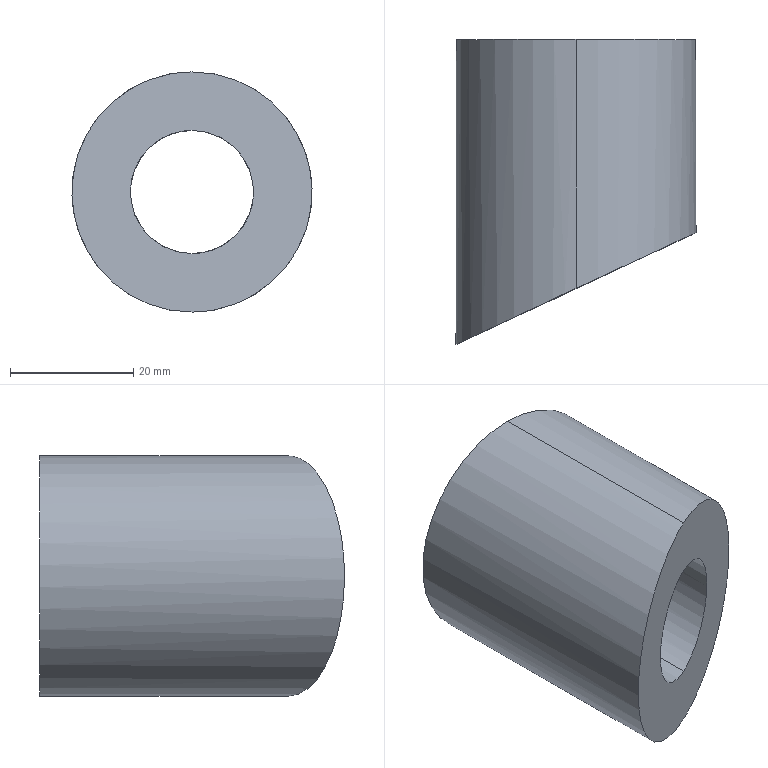Part | STEP file | PN_0016 Oil seal | 1 solid | 6 faces | box 39 x 49.525 x 39 mm | volume 35597 mm3 | cylinder 4 | plane 2 | commonest cylinder face diameters 20 x2 39 x2
STEP:
#1=CARTESIAN_POINT('',(0.,0.,0.));
#2=DIRECTION('',(0.,0.,1.));
#3=DIRECTION('',(1.,0.,0.));
#4=AXIS2_PLACEMENT_3D('',#1,#2,#3);
#5=CARTESIAN_POINT('',(0.,50.,-10.));
#6=VERTEX_POINT('',#5);
#7=CARTESIAN_POINT('',(0.,9.568,-10.));
#8=VERTEX_POINT('',#7);
#9=CARTESIAN_POINT('',(0.,50.,-10.));
#10=DIRECTION('',(0.,-1.,0.));
#11=VECTOR('',#10,1.);
#12=LINE('',#9,#11);
#13=CARTESIAN_POINT('',(0.,50.,0.));
#14=DIRECTION('',(0.,-1.,0.));
#15=DIRECTION('',(0.,0.,-1.));
#16=AXIS2_PLACEMENT_3D('',#13,#14,#15);
#17=CYLINDRICAL_SURFACE('',#16,10.);
#18=CARTESIAN_POINT('',(6.283,0.));
#19=DIRECTION('',(0.,1.));
#20=VECTOR('',#19,1.);
#21=LINE('',#18,#20);
#22=(GEOMETRIC_REPRESENTATION_CONTEXT(2)PARAMETRIC_REPRESENTATION_CONTEXT()REPRESENTATION_CONTEXT('',''));
#23=DEFINITIONAL_REPRESENTATION('',(#21),#22);
#24=PCURVE('',#17,#23);
#25=CARTESIAN_POINT('',(0.,50.,0.));
#26=DIRECTION('',(0.,-1.,0.));
#27=DIRECTION('',(0.,0.,-1.));
#28=AXIS2_PLACEMENT_3D('',#25,#26,#27);
#29=CYLINDRICAL_SURFACE('',#28,10.);
#30=CARTESIAN_POINT('',(0.,0.));
#31=DIRECTION('',(0.,1.));
#32=VECTOR('',#31,1.);
#33=LINE('',#30,#32);
#34=(GEOMETRIC_REPRESENTATION_CONTEXT(2)PARAMETRIC_REPRESENTATION_CONTEXT()REPRESENTATION_CONTEXT('',''));
#35=DEFINITIONAL_REPRESENTATION('',(#33),#34);
#36=PCURVE('',#29,#35);
#37=SURFACE_CURVE('',#12,(#24,#36),.PCURVE_S1.);
#38=EDGE_CURVE('',#6,#8,#37,.T.);
#39=ORIENTED_EDGE('',*,*,#38,.T.);
#40=CARTESIAN_POINT('',(0.,9.568,10.));
#41=VERTEX_POINT('',#40);
#42=CARTESIAN_POINT('',(0.,9.568,-10.));
#43=CARTESIAN_POINT('',(-20.,0.2419,-10.));
#44=CARTESIAN_POINT('',(-20.,0.2419,10.));
#45=CARTESIAN_POINT('',(0.,9.568,10.));
#46=(BOUNDED_CURVE()B_SPLINE_CURVE(3,(#42,#43,#44,#45),.UNSPECIFIED.,.F.,.F.)B_SPLINE_CURVE_WITH_KNOTS((4,4),(4.712,7.854),.PIECEWISE_BEZIER_KNOTS.)CURVE()GEOMETRIC_REPRESENTATION_ITEM()RATIONAL_B_SPLINE_CURVE((1.,0.3333,0.3333,1.))REPRESENTATION_ITEM(''));
#47=CARTESIAN_POINT('',(6.283,40.432));
#48=CARTESIAN_POINT('',(6.253,40.573));
#49=CARTESIAN_POINT('',(6.19,40.869));
#50=CARTESIAN_POINT('',(6.085,41.35));
#51=CARTESIAN_POINT('',(5.972,41.864));
#52=CARTESIAN_POINT('',(5.848,42.405));
#53=CARTESIAN_POINT('',(5.713,42.958));
#54=CARTESIAN_POINT('',(5.567,43.504));
#55=CARTESIAN_POINT('',(5.412,44.017));
#56=CARTESIAN_POINT('',(5.246,44.466));
#57=CARTESIAN_POINT('',(5.073,44.818));
#58=CARTESIAN_POINT('',(4.894,45.043));
#59=CARTESIAN_POINT('',(4.712,45.121));
#60=CARTESIAN_POINT('',(4.531,45.043));
#61=CARTESIAN_POINT('',(4.352,44.818));
#62=CARTESIAN_POINT('',(4.179,44.466));
#63=CARTESIAN_POINT('',(4.013,44.017));
#64=CARTESIAN_POINT('',(3.857,43.504));
#65=CARTESIAN_POINT('',(3.712,42.958));
#66=CARTESIAN_POINT('',(3.577,42.405));
#67=CARTESIAN_POINT('',(3.453,41.864));
#68=CARTESIAN_POINT('',(3.339,41.35));
#69=CARTESIAN_POINT('',(3.235,40.869));
#70=CARTESIAN_POINT('',(3.172,40.573));
#71=CARTESIAN_POINT('',(3.142,40.432));
#72=B_SPLINE_CURVE_WITH_KNOTS('',3,(#47,#48,#49,#50,#51,#52,#53,#54,#55,#56,#57,#58,#59,#60,#61,#62,#63,#64,#65,#66,#67,#68,#69,#70,#71),.UNSPECIFIED.,.F.,.F.,(4,1,1,1,1,1,1,1,1,1,1,1,1,1,1,1,1,1,1,1,1,1,4),(4.712,4.855,4.998,5.141,5.284,5.426,5.569,5.712,5.855,5.998,6.14,6.283,6.426,6.569,6.712,6.854,6.997,7.14,7.283,7.426,7.568,7.711,7.854),.QUASI_UNIFORM_KNOTS.);
#73=(GEOMETRIC_REPRESENTATION_CONTEXT(2)PARAMETRIC_REPRESENTATION_CONTEXT()REPRESENTATION_CONTEXT('',''));
#74=DEFINITIONAL_REPRESENTATION('',(#72),#73);
#75=PCURVE('',#17,#74);
#76=CARTESIAN_POINT('',(-103.019,-38.47,-30.));
#77=DIRECTION('',(-0.4226,0.9063,0.));
#78=DIRECTION('',(-0.9063,-0.4226,0.));
#79=AXIS2_PLACEMENT_3D('',#76,#77,#78);
#80=PLANE('',#79);
#81=CARTESIAN_POINT('',(-113.669,20.));
#82=CARTESIAN_POINT('',(-91.601,20.));
#83=CARTESIAN_POINT('',(-91.601,40.));
#84=CARTESIAN_POINT('',(-113.669,40.));
#85=(BOUNDED_CURVE()B_SPLINE_CURVE(3,(#81,#82,#83,#84),.UNSPECIFIED.,.F.,.F.)B_SPLINE_CURVE_WITH_KNOTS((4,4),(4.712,7.854),.PIECEWISE_BEZIER_KNOTS.)CURVE()GEOMETRIC_REPRESENTATION_ITEM()RATIONAL_B_SPLINE_CURVE((1.,0.3333,0.3333,1.))REPRESENTATION_ITEM(''));
#86=(GEOMETRIC_REPRESENTATION_CONTEXT(2)PARAMETRIC_REPRESENTATION_CONTEXT()REPRESENTATION_CONTEXT('',''));
#87=DEFINITIONAL_REPRESENTATION('',(#85),#86);
#88=PCURVE('',#80,#87);
#89=SURFACE_CURVE('',#46,(#75,#88),.PCURVE_S1.);
#90=EDGE_CURVE('',#8,#41,#89,.T.);
#91=ORIENTED_EDGE('',*,*,#90,.T.);
#92=CARTESIAN_POINT('',(0.,50.,10.));
#93=VERTEX_POINT('',#92);
#94=CARTESIAN_POINT('',(0.,50.,10.));
#95=DIRECTION('',(0.,-1.,0.));
#96=VECTOR('',#95,1.);
#97=LINE('',#94,#96);
#98=CARTESIAN_POINT('',(3.142,0.));
#99=DIRECTION('',(0.,1.));
#100=VECTOR('',#99,1.);
#101=LINE('',#98,#100);
#102=(GEOMETRIC_REPRESENTATION_CONTEXT(2)PARAMETRIC_REPRESENTATION_CONTEXT()REPRESENTATION_CONTEXT('',''));
#103=DEFINITIONAL_REPRESENTATION('',(#101),#102);
#104=PCURVE('',#17,#103);
#105=CARTESIAN_POINT('',(3.142,0.));
#106=DIRECTION('',(0.,1.));
#107=VECTOR('',#106,1.);
#108=LINE('',#105,#107);
#109=(GEOMETRIC_REPRESENTATION_CONTEXT(2)PARAMETRIC_REPRESENTATION_CONTEXT()REPRESENTATION_CONTEXT('',''));
#110=DEFINITIONAL_REPRESENTATION('',(#108),#109);
#111=PCURVE('',#29,#110);
#112=SURFACE_CURVE('',#97,(#104,#111),.PCURVE_S1.);
#113=EDGE_CURVE('',#93,#41,#112,.T.);
#114=ORIENTED_EDGE('',*,*,#113,.F.);
#115=CARTESIAN_POINT('',(0.,50.,0.));
#116=DIRECTION('',(0.,1.,0.));
#117=DIRECTION('',(0.,0.,1.));
#118=AXIS2_PLACEMENT_3D('',#115,#116,#117);
#119=CIRCLE('',#118,10.);
#120=CARTESIAN_POINT('',(9.425,0.));
#121=DIRECTION('',(-1.,0.));
#122=VECTOR('',#121,1.);
#123=LINE('',#120,#122);
#124=(GEOMETRIC_REPRESENTATION_CONTEXT(2)PARAMETRIC_REPRESENTATION_CONTEXT()REPRESENTATION_CONTEXT('',''));
#125=DEFINITIONAL_REPRESENTATION('',(#123),#124);
#126=PCURVE('',#17,#125);
#127=CARTESIAN_POINT('',(0.,50.,0.));
#128=DIRECTION('',(0.,1.,0.));
#129=DIRECTION('',(0.,0.,1.));
#130=AXIS2_PLACEMENT_3D('',#127,#128,#129);
#131=PLANE('',#130);
#132=CARTESIAN_POINT('',(0.,0.));
#133=DIRECTION('',(1.,0.));
#134=AXIS2_PLACEMENT_2D('',#132,#133);
#135=CIRCLE('',#134,10.);
#136=(GEOMETRIC_REPRESENTATION_CONTEXT(2)PARAMETRIC_REPRESENTATION_CONTEXT()REPRESENTATION_CONTEXT('',''));
#137=DEFINITIONAL_REPRESENTATION('',(#135),#136);
#138=PCURVE('',#131,#137);
#139=SURFACE_CURVE('',#119,(#126,#138),.PCURVE_S1.);
#140=EDGE_CURVE('',#6,#93,#139,.T.);
#141=ORIENTED_EDGE('',*,*,#140,.F.);
#142=EDGE_LOOP('',(#39,#91,#114,#141));
#143=FACE_BOUND('',#142,.F.);
#144=ADVANCED_FACE('',(#143),#17,.F.);
#145=CARTESIAN_POINT('',(0.,50.,19.5));
#146=VERTEX_POINT('',#145);
#147=CARTESIAN_POINT('',(0.,50.,-19.5));
#148=VERTEX_POINT('',#147);
#149=CARTESIAN_POINT('',(0.,50.,0.));
#150=DIRECTION('',(0.,1.,0.));
#151=DIRECTION('',(0.,0.,1.));
#152=AXIS2_PLACEMENT_3D('',#149,#150,#151);
#153=CIRCLE('',#152,19.5);
#154=CARTESIAN_POINT('',(0.,50.,0.));
#155=DIRECTION('',(0.,-1.,0.));
#156=DIRECTION('',(0.,0.,-1.));
#157=AXIS2_PLACEMENT_3D('',#154,#155,#156);
#158=CYLINDRICAL_SURFACE('',#157,19.5);
#159=CARTESIAN_POINT('',(3.142,0.));
#160=DIRECTION('',(-1.,0.));
#161=VECTOR('',#160,1.);
#162=LINE('',#159,#161);
#163=(GEOMETRIC_REPRESENTATION_CONTEXT(2)PARAMETRIC_REPRESENTATION_CONTEXT()REPRESENTATION_CONTEXT('',''));
#164=DEFINITIONAL_REPRESENTATION('',(#162),#163);
#165=PCURVE('',#158,#164);
#166=CARTESIAN_POINT('',(0.,0.));
#167=DIRECTION('',(1.,0.));
#168=AXIS2_PLACEMENT_2D('',#166,#167);
#169=CIRCLE('',#168,19.5);
#170=(GEOMETRIC_REPRESENTATION_CONTEXT(2)PARAMETRIC_REPRESENTATION_CONTEXT()REPRESENTATION_CONTEXT('',''));
#171=DEFINITIONAL_REPRESENTATION('',(#169),#170);
#172=PCURVE('',#131,#171);
#173=SURFACE_CURVE('',#153,(#165,#172),.PCURVE_S1.);
#174=EDGE_CURVE('',#146,#148,#173,.T.);
#175=ORIENTED_EDGE('',*,*,#174,.F.);
#176=CARTESIAN_POINT('',(0.,9.568,19.5));
#177=VERTEX_POINT('',#176);
#178=CARTESIAN_POINT('',(0.,50.,19.5));
#179=DIRECTION('',(0.,-1.,0.));
#180=VECTOR('',#179,1.);
#181=LINE('',#178,#180);
#182=CARTESIAN_POINT('',(3.142,0.));
#183=DIRECTION('',(0.,1.));
#184=VECTOR('',#183,1.);
#185=LINE('',#182,#184);
#186=(GEOMETRIC_REPRESENTATION_CONTEXT(2)PARAMETRIC_REPRESENTATION_CONTEXT()REPRESENTATION_CONTEXT('',''));
#187=DEFINITIONAL_REPRESENTATION('',(#185),#186);
#188=PCURVE('',#158,#187);
#189=CARTESIAN_POINT('',(0.,50.,0.));
#190=DIRECTION('',(0.,-1.,0.));
#191=DIRECTION('',(0.,0.,-1.));
#192=AXIS2_PLACEMENT_3D('',#189,#190,#191);
#193=CYLINDRICAL_SURFACE('',#192,19.5);
#194=CARTESIAN_POINT('',(3.142,0.));
#195=DIRECTION('',(0.,1.));
#196=VECTOR('',#195,1.);
#197=LINE('',#194,#196);
#198=(GEOMETRIC_REPRESENTATION_CONTEXT(2)PARAMETRIC_REPRESENTATION_CONTEXT()REPRESENTATION_CONTEXT('',''));
#199=DEFINITIONAL_REPRESENTATION('',(#197),#198);
#200=PCURVE('',#193,#199);
#201=SURFACE_CURVE('',#181,(#188,#200),.PCURVE_S1.);
#202=EDGE_CURVE('',#146,#177,#201,.T.);
#203=ORIENTED_EDGE('',*,*,#202,.T.);
#204=CARTESIAN_POINT('',(0.,9.568,-19.5));
#205=VERTEX_POINT('',#204);
#206=CARTESIAN_POINT('',(0.,9.568,19.5));
#207=CARTESIAN_POINT('',(39.,27.754,19.5));
#208=CARTESIAN_POINT('',(39.,27.754,-19.5));
#209=CARTESIAN_POINT('',(0.,9.568,-19.5));
#210=(BOUNDED_CURVE()B_SPLINE_CURVE(3,(#206,#207,#208,#209),.UNSPECIFIED.,.F.,.F.)B_SPLINE_CURVE_WITH_KNOTS((4,4),(1.571,4.712),.PIECEWISE_BEZIER_KNOTS.)CURVE()GEOMETRIC_REPRESENTATION_ITEM()RATIONAL_B_SPLINE_CURVE((1.,0.3333,0.3333,1.))REPRESENTATION_ITEM(''));
#211=CARTESIAN_POINT('',(3.142,40.432));
#212=CARTESIAN_POINT('',(3.111,40.157));
#213=CARTESIAN_POINT('',(3.048,39.58));
#214=CARTESIAN_POINT('',(2.944,38.642));
#215=CARTESIAN_POINT('',(2.83,37.639));
#216=CARTESIAN_POINT('',(2.706,36.585));
#217=CARTESIAN_POINT('',(2.571,35.507));
#218=CARTESIAN_POINT('',(2.426,34.442));
#219=CARTESIAN_POINT('',(2.27,33.442));
#220=CARTESIAN_POINT('',(2.105,32.567));
#221=CARTESIAN_POINT('',(1.931,31.88));
#222=CARTESIAN_POINT('',(1.753,31.44));
#223=CARTESIAN_POINT('',(1.571,31.288));
#224=CARTESIAN_POINT('',(1.389,31.44));
#225=CARTESIAN_POINT('',(1.21,31.88));
#226=CARTESIAN_POINT('',(1.037,32.567));
#227=CARTESIAN_POINT('',(0.8717,33.442));
#228=CARTESIAN_POINT('',(0.7158,34.442));
#229=CARTESIAN_POINT('',(0.5703,35.507));
#230=CARTESIAN_POINT('',(0.4356,36.585));
#231=CARTESIAN_POINT('',(0.3115,37.639));
#232=CARTESIAN_POINT('',(0.1977,38.642));
#233=CARTESIAN_POINT('',(0.09367,39.58));
#234=CARTESIAN_POINT('',(0.0303,40.157));
#235=CARTESIAN_POINT('',(0.,40.432));
#236=B_SPLINE_CURVE_WITH_KNOTS('',3,(#211,#212,#213,#214,#215,#216,#217,#218,#219,#220,#221,#222,#223,#224,#225,#226,#227,#228,#229,#230,#231,#232,#233,#234,#235),.UNSPECIFIED.,.F.,.F.,(4,1,1,1,1,1,1,1,1,1,1,1,1,1,1,1,1,1,1,1,1,1,4),(1.571,1.714,1.856,1.999,2.142,2.285,2.428,2.57,2.713,2.856,2.999,3.142,3.284,3.427,3.57,3.713,3.856,3.998,4.141,4.284,4.427,4.57,4.712),.QUASI_UNIFORM_KNOTS.);
#237=(GEOMETRIC_REPRESENTATION_CONTEXT(2)PARAMETRIC_REPRESENTATION_CONTEXT()REPRESENTATION_CONTEXT('',''));
#238=DEFINITIONAL_REPRESENTATION('',(#236),#237);
#239=PCURVE('',#158,#238);
#240=CARTESIAN_POINT('',(-113.669,49.5));
#241=CARTESIAN_POINT('',(-156.7,49.5));
#242=CARTESIAN_POINT('',(-156.7,10.5));
#243=CARTESIAN_POINT('',(-113.669,10.5));
#244=(BOUNDED_CURVE()B_SPLINE_CURVE(3,(#240,#241,#242,#243),.UNSPECIFIED.,.F.,.F.)B_SPLINE_CURVE_WITH_KNOTS((4,4),(1.571,4.712),.PIECEWISE_BEZIER_KNOTS.)CURVE()GEOMETRIC_REPRESENTATION_ITEM()RATIONAL_B_SPLINE_CURVE((1.,0.3333,0.3333,1.))REPRESENTATION_ITEM(''));
#245=(GEOMETRIC_REPRESENTATION_CONTEXT(2)PARAMETRIC_REPRESENTATION_CONTEXT()REPRESENTATION_CONTEXT('',''));
#246=DEFINITIONAL_REPRESENTATION('',(#244),#245);
#247=PCURVE('',#80,#246);
#248=SURFACE_CURVE('',#210,(#239,#247),.PCURVE_S1.);
#249=EDGE_CURVE('',#177,#205,#248,.T.);
#250=ORIENTED_EDGE('',*,*,#249,.T.);
#251=CARTESIAN_POINT('',(0.,50.,-19.5));
#252=DIRECTION('',(0.,-1.,0.));
#253=VECTOR('',#252,1.);
#254=LINE('',#251,#253);
#255=CARTESIAN_POINT('',(0.,0.));
#256=DIRECTION('',(0.,1.));
#257=VECTOR('',#256,1.);
#258=LINE('',#255,#257);
#259=(GEOMETRIC_REPRESENTATION_CONTEXT(2)PARAMETRIC_REPRESENTATION_CONTEXT()REPRESENTATION_CONTEXT('',''));
#260=DEFINITIONAL_REPRESENTATION('',(#258),#259);
#261=PCURVE('',#158,#260);
#262=CARTESIAN_POINT('',(6.283,0.));
#263=DIRECTION('',(0.,1.));
#264=VECTOR('',#263,1.);
#265=LINE('',#262,#264);
#266=(GEOMETRIC_REPRESENTATION_CONTEXT(2)PARAMETRIC_REPRESENTATION_CONTEXT()REPRESENTATION_CONTEXT('',''));
#267=DEFINITIONAL_REPRESENTATION('',(#265),#266);
#268=PCURVE('',#193,#267);
#269=SURFACE_CURVE('',#254,(#261,#268),.PCURVE_S1.);
#270=EDGE_CURVE('',#148,#205,#269,.T.);
#271=ORIENTED_EDGE('',*,*,#270,.F.);
#272=EDGE_LOOP('',(#175,#203,#250,#271));
#273=FACE_BOUND('',#272,.T.);
#274=ADVANCED_FACE('',(#273),#158,.T.);
#275=CARTESIAN_POINT('',(0.,50.,0.));
#276=DIRECTION('',(0.,1.,0.));
#277=DIRECTION('',(0.,0.,1.));
#278=AXIS2_PLACEMENT_3D('',#275,#276,#277);
#279=CIRCLE('',#278,19.5);
#280=CARTESIAN_POINT('',(0.,0.));
#281=DIRECTION('',(1.,0.));
#282=AXIS2_PLACEMENT_2D('',#280,#281);
#283=CIRCLE('',#282,19.5);
#284=(GEOMETRIC_REPRESENTATION_CONTEXT(2)PARAMETRIC_REPRESENTATION_CONTEXT()REPRESENTATION_CONTEXT('',''));
#285=DEFINITIONAL_REPRESENTATION('',(#283),#284);
#286=PCURVE('',#131,#285);
#287=CARTESIAN_POINT('',(9.425,0.));
#288=DIRECTION('',(-1.,0.));
#289=VECTOR('',#288,1.);
#290=LINE('',#287,#289);
#291=(GEOMETRIC_REPRESENTATION_CONTEXT(2)PARAMETRIC_REPRESENTATION_CONTEXT()REPRESENTATION_CONTEXT('',''));
#292=DEFINITIONAL_REPRESENTATION('',(#290),#291);
#293=PCURVE('',#193,#292);
#294=SURFACE_CURVE('',#279,(#286,#293),.PCURVE_S1.);
#295=EDGE_CURVE('',#148,#146,#294,.T.);
#296=ORIENTED_EDGE('',*,*,#295,.T.);
#297=ORIENTED_EDGE('',*,*,#174,.T.);
#298=EDGE_LOOP('',(#296,#297));
#299=FACE_BOUND('',#298,.T.);
#300=ORIENTED_EDGE('',*,*,#140,.F.);
#301=CARTESIAN_POINT('',(0.,50.,0.));
#302=DIRECTION('',(0.,1.,0.));
#303=DIRECTION('',(0.,0.,1.));
#304=AXIS2_PLACEMENT_3D('',#301,#302,#303);
#305=CIRCLE('',#304,10.);
#306=CARTESIAN_POINT('',(0.,0.));
#307=DIRECTION('',(1.,0.));
#308=AXIS2_PLACEMENT_2D('',#306,#307);
#309=CIRCLE('',#308,10.);
#310=(GEOMETRIC_REPRESENTATION_CONTEXT(2)PARAMETRIC_REPRESENTATION_CONTEXT()REPRESENTATION_CONTEXT('',''));
#311=DEFINITIONAL_REPRESENTATION('',(#309),#310);
#312=PCURVE('',#131,#311);
#313=CARTESIAN_POINT('',(3.142,0.));
#314=DIRECTION('',(-1.,0.));
#315=VECTOR('',#314,1.);
#316=LINE('',#313,#315);
#317=(GEOMETRIC_REPRESENTATION_CONTEXT(2)PARAMETRIC_REPRESENTATION_CONTEXT()REPRESENTATION_CONTEXT('',''));
#318=DEFINITIONAL_REPRESENTATION('',(#316),#317);
#319=PCURVE('',#29,#318);
#320=SURFACE_CURVE('',#305,(#312,#319),.PCURVE_S1.);
#321=EDGE_CURVE('',#93,#6,#320,.T.);
#322=ORIENTED_EDGE('',*,*,#321,.F.);
#323=EDGE_LOOP('',(#300,#322));
#324=FACE_BOUND('',#323,.T.);
#325=ADVANCED_FACE('',(#299,#324),#131,.T.);
#326=ORIENTED_EDGE('',*,*,#202,.F.);
#327=ORIENTED_EDGE('',*,*,#295,.F.);
#328=ORIENTED_EDGE('',*,*,#270,.T.);
#329=CARTESIAN_POINT('',(0.,9.568,-19.5));
#330=CARTESIAN_POINT('',(-39.,-8.618,-19.5));
#331=CARTESIAN_POINT('',(-39.,-8.618,19.5));
#332=CARTESIAN_POINT('',(0.,9.568,19.5));
#333=(BOUNDED_CURVE()B_SPLINE_CURVE(3,(#329,#330,#331,#332),.UNSPECIFIED.,.F.,.F.)B_SPLINE_CURVE_WITH_KNOTS((4,4),(4.712,7.854),.PIECEWISE_BEZIER_KNOTS.)CURVE()GEOMETRIC_REPRESENTATION_ITEM()RATIONAL_B_SPLINE_CURVE((1.,0.3333,0.3333,1.))REPRESENTATION_ITEM(''));
#334=CARTESIAN_POINT('',(6.283,40.432));
#335=CARTESIAN_POINT('',(6.253,40.707));
#336=CARTESIAN_POINT('',(6.19,41.284));
#337=CARTESIAN_POINT('',(6.085,42.222));
#338=CARTESIAN_POINT('',(5.972,43.225));
#339=CARTESIAN_POINT('',(5.848,44.279));
#340=CARTESIAN_POINT('',(5.713,45.357));
#341=CARTESIAN_POINT('',(5.567,46.422));
#342=CARTESIAN_POINT('',(5.412,47.422));
#343=CARTESIAN_POINT('',(5.246,48.297));
#344=CARTESIAN_POINT('',(5.073,48.984));
#345=CARTESIAN_POINT('',(4.894,49.424));
#346=CARTESIAN_POINT('',(4.712,49.575));
#347=CARTESIAN_POINT('',(4.531,49.424));
#348=CARTESIAN_POINT('',(4.352,48.984));
#349=CARTESIAN_POINT('',(4.179,48.297));
#350=CARTESIAN_POINT('',(4.013,47.422));
#351=CARTESIAN_POINT('',(3.857,46.422));
#352=CARTESIAN_POINT('',(3.712,45.357));
#353=CARTESIAN_POINT('',(3.577,44.279));
#354=CARTESIAN_POINT('',(3.453,43.225));
#355=CARTESIAN_POINT('',(3.339,42.222));
#356=CARTESIAN_POINT('',(3.235,41.284));
#357=CARTESIAN_POINT('',(3.172,40.707));
#358=CARTESIAN_POINT('',(3.142,40.432));
#359=B_SPLINE_CURVE_WITH_KNOTS('',3,(#334,#335,#336,#337,#338,#339,#340,#341,#342,#343,#344,#345,#346,#347,#348,#349,#350,#351,#352,#353,#354,#355,#356,#357,#358),.UNSPECIFIED.,.F.,.F.,(4,1,1,1,1,1,1,1,1,1,1,1,1,1,1,1,1,1,1,1,1,1,4),(4.712,4.855,4.998,5.141,5.284,5.426,5.569,5.712,5.855,5.998,6.14,6.283,6.426,6.569,6.712,6.854,6.997,7.14,7.283,7.426,7.568,7.711,7.854),.QUASI_UNIFORM_KNOTS.);
#360=(GEOMETRIC_REPRESENTATION_CONTEXT(2)PARAMETRIC_REPRESENTATION_CONTEXT()REPRESENTATION_CONTEXT('',''));
#361=DEFINITIONAL_REPRESENTATION('',(#359),#360);
#362=PCURVE('',#193,#361);
#363=CARTESIAN_POINT('',(-113.669,10.5));
#364=CARTESIAN_POINT('',(-70.637,10.5));
#365=CARTESIAN_POINT('',(-70.637,49.5));
#366=CARTESIAN_POINT('',(-113.669,49.5));
#367=(BOUNDED_CURVE()B_SPLINE_CURVE(3,(#363,#364,#365,#366),.UNSPECIFIED.,.F.,.F.)B_SPLINE_CURVE_WITH_KNOTS((4,4),(4.712,7.854),.PIECEWISE_BEZIER_KNOTS.)CURVE()GEOMETRIC_REPRESENTATION_ITEM()RATIONAL_B_SPLINE_CURVE((1.,0.3333,0.3333,1.))REPRESENTATION_ITEM(''));
#368=(GEOMETRIC_REPRESENTATION_CONTEXT(2)PARAMETRIC_REPRESENTATION_CONTEXT()REPRESENTATION_CONTEXT('',''));
#369=DEFINITIONAL_REPRESENTATION('',(#367),#368);
#370=PCURVE('',#80,#369);
#371=SURFACE_CURVE('',#333,(#362,#370),.PCURVE_S1.);
#372=EDGE_CURVE('',#205,#177,#371,.T.);
#373=ORIENTED_EDGE('',*,*,#372,.T.);
#374=EDGE_LOOP('',(#326,#327,#328,#373));
#375=FACE_BOUND('',#374,.T.);
#376=ADVANCED_FACE('',(#375),#193,.T.);
#377=CARTESIAN_POINT('',(0.,9.568,10.));
#378=CARTESIAN_POINT('',(20.,18.894,10.));
#379=CARTESIAN_POINT('',(20.,18.894,-10.));
#380=CARTESIAN_POINT('',(0.,9.568,-10.));
#381=(BOUNDED_CURVE()B_SPLINE_CURVE(3,(#377,#378,#379,#380),.UNSPECIFIED.,.F.,.F.)B_SPLINE_CURVE_WITH_KNOTS((4,4),(1.571,4.712),.PIECEWISE_BEZIER_KNOTS.)CURVE()GEOMETRIC_REPRESENTATION_ITEM()RATIONAL_B_SPLINE_CURVE((1.,0.3333,0.3333,1.))REPRESENTATION_ITEM(''));
#382=CARTESIAN_POINT('',(3.142,40.432));
#383=CARTESIAN_POINT('',(3.111,40.291));
#384=CARTESIAN_POINT('',(3.048,39.995));
#385=CARTESIAN_POINT('',(2.944,39.514));
#386=CARTESIAN_POINT('',(2.83,39.));
#387=CARTESIAN_POINT('',(2.706,38.459));
#388=CARTESIAN_POINT('',(2.571,37.906));
#389=CARTESIAN_POINT('',(2.426,37.36));
#390=CARTESIAN_POINT('',(2.27,36.847));
#391=CARTESIAN_POINT('',(2.105,36.398));
#392=CARTESIAN_POINT('',(1.931,36.046));
#393=CARTESIAN_POINT('',(1.753,35.821));
#394=CARTESIAN_POINT('',(1.571,35.743));
#395=CARTESIAN_POINT('',(1.389,35.821));
#396=CARTESIAN_POINT('',(1.21,36.046));
#397=CARTESIAN_POINT('',(1.037,36.398));
#398=CARTESIAN_POINT('',(0.8717,36.847));
#399=CARTESIAN_POINT('',(0.7158,37.36));
#400=CARTESIAN_POINT('',(0.5703,37.906));
#401=CARTESIAN_POINT('',(0.4356,38.459));
#402=CARTESIAN_POINT('',(0.3115,39.));
#403=CARTESIAN_POINT('',(0.1977,39.514));
#404=CARTESIAN_POINT('',(0.09367,39.995));
#405=CARTESIAN_POINT('',(0.0303,40.291));
#406=CARTESIAN_POINT('',(0.,40.432));
#407=B_SPLINE_CURVE_WITH_KNOTS('',3,(#382,#383,#384,#385,#386,#387,#388,#389,#390,#391,#392,#393,#394,#395,#396,#397,#398,#399,#400,#401,#402,#403,#404,#405,#406),.UNSPECIFIED.,.F.,.F.,(4,1,1,1,1,1,1,1,1,1,1,1,1,1,1,1,1,1,1,1,1,1,4),(1.571,1.714,1.856,1.999,2.142,2.285,2.428,2.57,2.713,2.856,2.999,3.142,3.284,3.427,3.57,3.713,3.856,3.998,4.141,4.284,4.427,4.57,4.712),.QUASI_UNIFORM_KNOTS.);
#408=(GEOMETRIC_REPRESENTATION_CONTEXT(2)PARAMETRIC_REPRESENTATION_CONTEXT()REPRESENTATION_CONTEXT('',''));
#409=DEFINITIONAL_REPRESENTATION('',(#407),#408);
#410=PCURVE('',#29,#409);
#411=CARTESIAN_POINT('',(-113.669,40.));
#412=CARTESIAN_POINT('',(-135.736,40.));
#413=CARTESIAN_POINT('',(-135.736,20.));
#414=CARTESIAN_POINT('',(-113.669,20.));
#415=(BOUNDED_CURVE()B_SPLINE_CURVE(3,(#411,#412,#413,#414),.UNSPECIFIED.,.F.,.F.)B_SPLINE_CURVE_WITH_KNOTS((4,4),(1.571,4.712),.PIECEWISE_BEZIER_KNOTS.)CURVE()GEOMETRIC_REPRESENTATION_ITEM()RATIONAL_B_SPLINE_CURVE((1.,0.3333,0.3333,1.))REPRESENTATION_ITEM(''));
#416=(GEOMETRIC_REPRESENTATION_CONTEXT(2)PARAMETRIC_REPRESENTATION_CONTEXT()REPRESENTATION_CONTEXT('',''));
#417=DEFINITIONAL_REPRESENTATION('',(#415),#416);
#418=PCURVE('',#80,#417);
#419=SURFACE_CURVE('',#381,(#410,#418),.PCURVE_S1.);
#420=EDGE_CURVE('',#41,#8,#419,.T.);
#421=ORIENTED_EDGE('',*,*,#420,.T.);
#422=ORIENTED_EDGE('',*,*,#38,.F.);
#423=ORIENTED_EDGE('',*,*,#321,.F.);
#424=ORIENTED_EDGE('',*,*,#113,.T.);
#425=EDGE_LOOP('',(#421,#422,#423,#424));
#426=FACE_BOUND('',#425,.F.);
#427=ADVANCED_FACE('',(#426),#29,.F.);
#428=ORIENTED_EDGE('',*,*,#90,.T.);
#429=ORIENTED_EDGE('',*,*,#420,.T.);
#430=EDGE_LOOP('',(#428,#429));
#431=FACE_BOUND('',#430,.T.);
#432=ORIENTED_EDGE('',*,*,#372,.F.);
#433=ORIENTED_EDGE('',*,*,#249,.F.);
#434=EDGE_LOOP('',(#432,#433));
#435=FACE_BOUND('',#434,.T.);
#436=ADVANCED_FACE('',(#431,#435),#80,.F.);
#437=CLOSED_SHELL('',(#144,#274,#325,#376,#427,#436));
#438=MANIFOLD_SOLID_BREP('',#437);
#439=(LENGTH_UNIT()NAMED_UNIT(*)SI_UNIT(.MILLI.,.METRE.));
#440=UNCERTAINTY_MEASURE_WITH_UNIT(LENGTH_MEASURE(0.0000001),#439,'','');
#441=(NAMED_UNIT(*)PLANE_ANGLE_UNIT()SI_UNIT($,.RADIAN.));
#442=(NAMED_UNIT(*)SI_UNIT($,.STERADIAN.)SOLID_ANGLE_UNIT());
#443=(GEOMETRIC_REPRESENTATION_CONTEXT(3)GLOBAL_UNCERTAINTY_ASSIGNED_CONTEXT((#440))GLOBAL_UNIT_ASSIGNED_CONTEXT((#439,#441,#442))REPRESENTATION_CONTEXT('',''));
#444=ADVANCED_BREP_SHAPE_REPRESENTATION('',(#4,#438),#443);